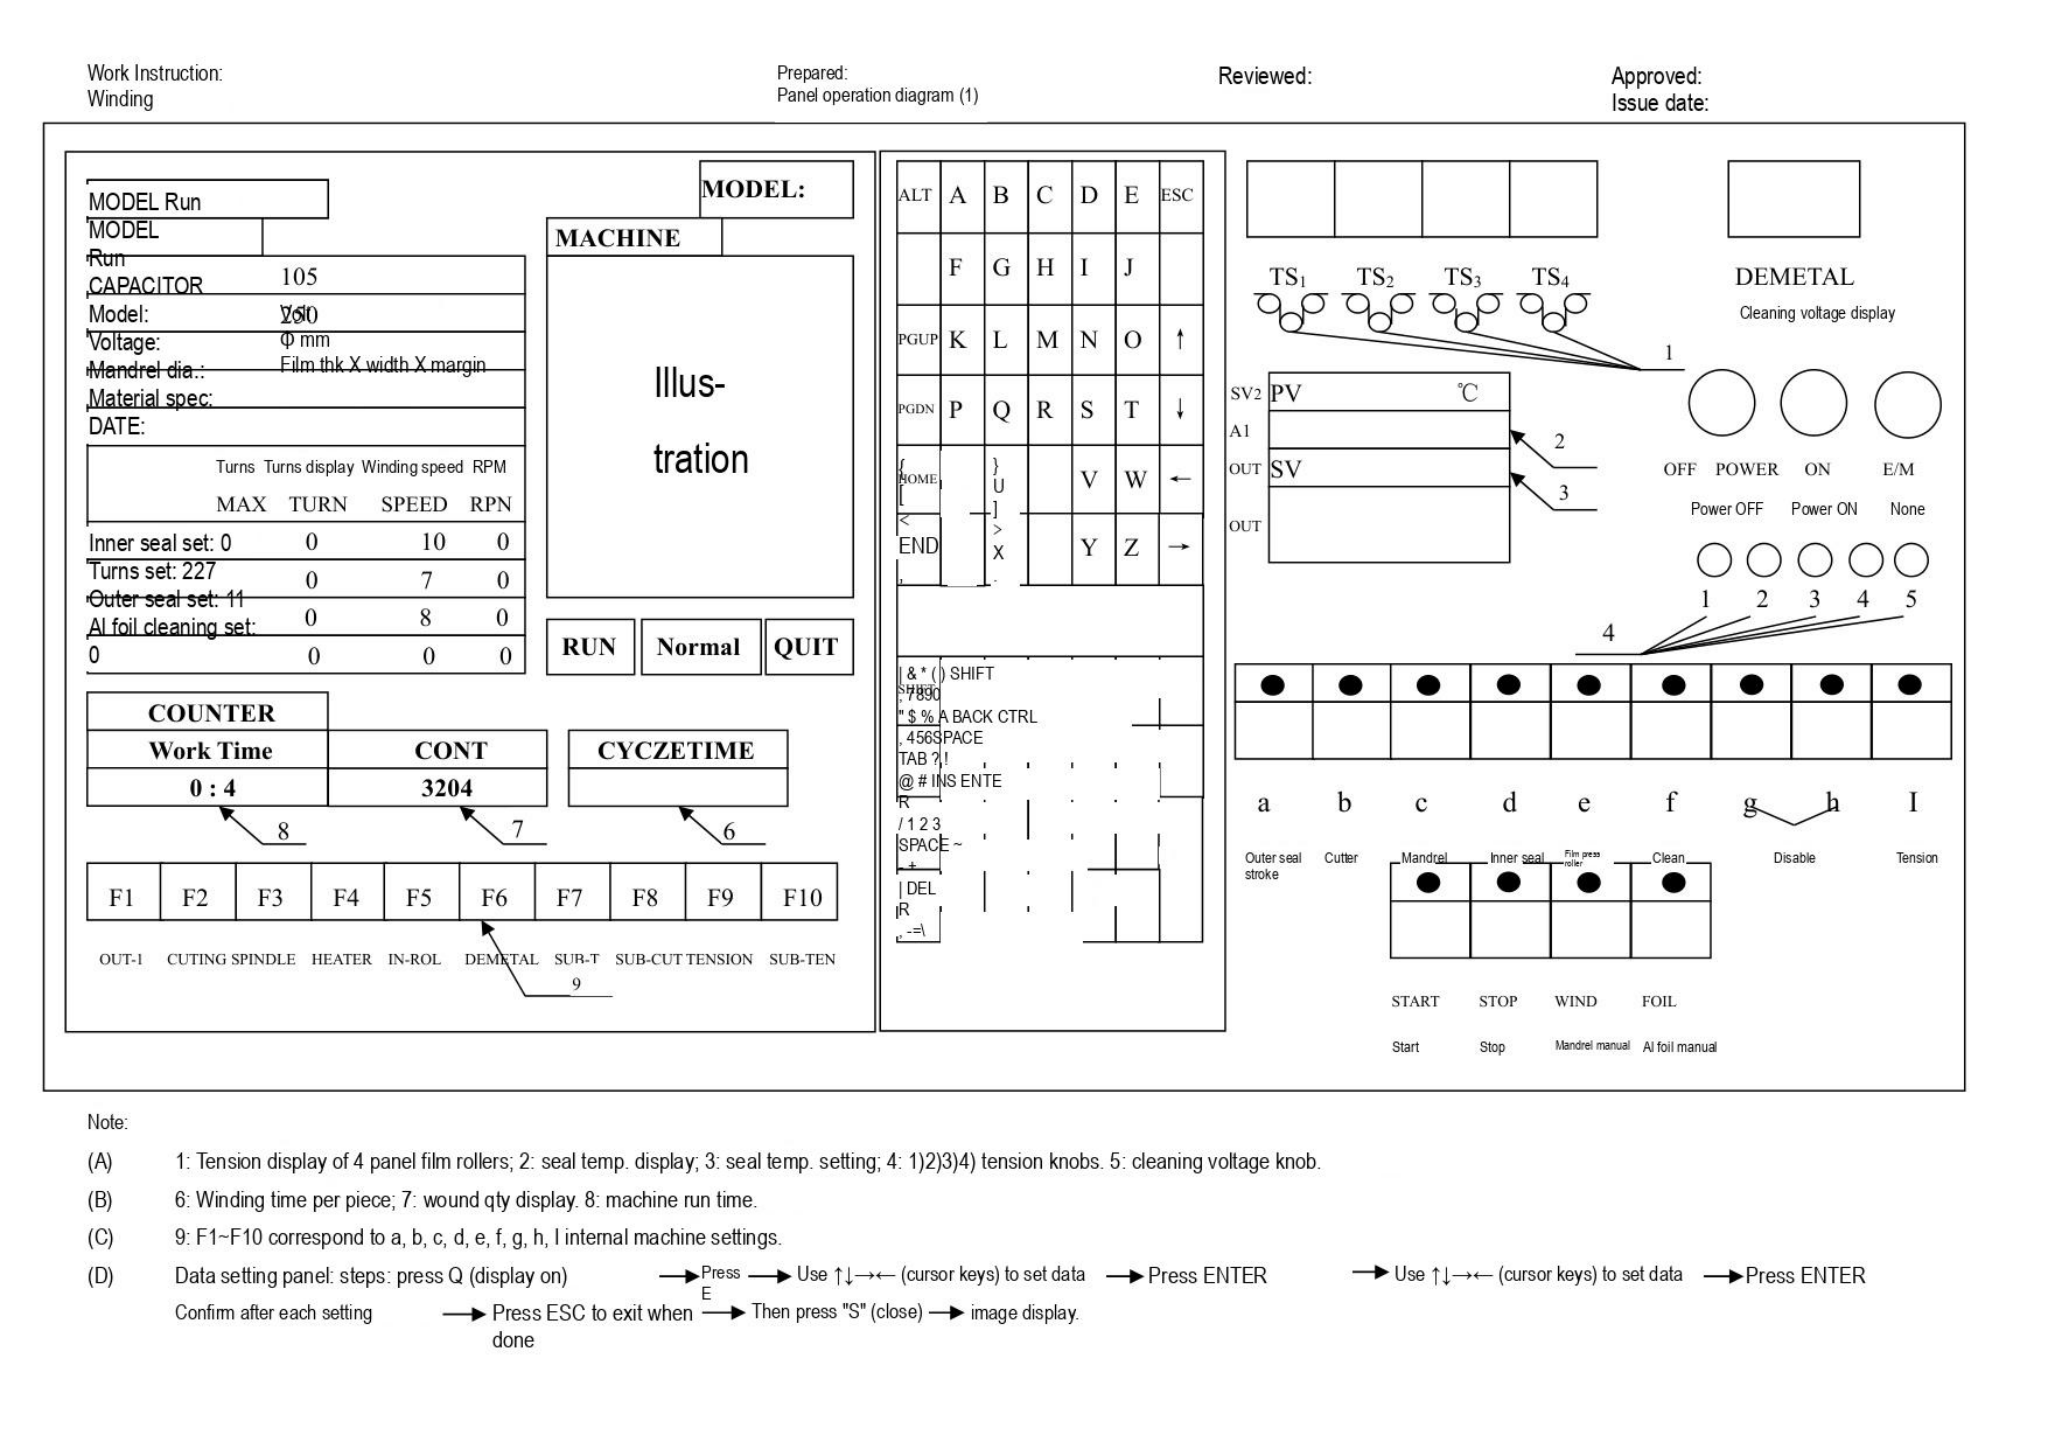Work Instruction:
Winding

Prepared:
Panel operation diagram (1)

Reviewed:

Approved:
Issue date:

MODEL Run
MODEL
Run

| | |
|---|---|
| CAPACITOR | 105 |
| Model: | 250 |
| Voltage: | Φ mm |
| Mandrel dia.: | Film thk X width X margin |
| Material spec: | |
| DATE: | |

| Turns | Turns display | Winding speed | RPM |
|---|---|---|---|
| MAX | TURN | SPEED | RPN |
| Inner seal set: 0 | 0 | 10 | 0 |
| Turns set: 227 | 0 | 7 | 0 |
| Outer seal set: 11 | 0 | 8 | 0 |
| Al foil cleaning set: | 0 | 0 | 0 |
| 0 | | | |

MODEL:

MACHINE

Illus-
tration

RUN Normal QUIT

| COUNTER | | |
|---|---|---|
| Work Time | CONT | CYCZETIME |
| 0 : 4 | 3204 | |

8 7 6

| F1 | F2 | F3 | F4 | F5 | F6 | F7 | F8 | F9 | F10 |
|---|---|---|---|---|---|---|---|---|---|

OUT-1 CUTING SPINDLE HEATER IN-ROL DEMETAL SUB-T SUB-CUT TENSION SUB-TEN

9

| ALT | A | B | C | D | E | ESC |
|---|---|---|---|---|---|---|
| | F | G | H | I | J | |
| PGUP | K | L | M | N | O | ↑ |
| PGDN | P | Q | R | S | T | ↓ |
| { HOME [ | | } U ] | | V | W | ← |
| < END | | > X | | Y | Z | → |

| & * ( ) SHIFT
SHIFT
, / 890
" $ % A BACK CTRL
, 456SPACE
TAB ? !
@ # INS ENTE
R
/ 1 2 3
SPACE ~
_ +
| DEL
R
. -=\

TS1 TS2 TS3 TS4

1

DEMETAL
Cleaning voltage display

SV2 PV ℃
A1
OUT SV
OUT

2
3

OFF POWER ON E/M
Power OFF Power ON None

1 2 3 4 5

4

a b c d e f g h I

Outer seal stroke | Cutter | Mandrel | Inner seal | Film press roller | Clean | Disable | Tension

START STOP WIND FOIL
Start Stop Mandrel manual Al foil manual

Note:

(A) 1: Tension display of 4 panel film rollers; 2: seal temp. display; 3: seal temp. setting; 4: 1)2)3)4) tension knobs. 5: cleaning voltage knob.

(B) 6: Winding time per piece; 7: wound qty display. 8: machine run time.

(C) 9: F1~F10 correspond to a, b, c, d, e, f, g, h, I internal machine settings.

(D) Data setting panel: steps: press Q (display on) → Press E → Use ↑↓→← (cursor keys) to set data → Press ENTER → Use ↑↓→← (cursor keys) to set data → Press ENTER
Confirm after each setting → Press ESC to exit when done → Then press "S" (close) → image display.
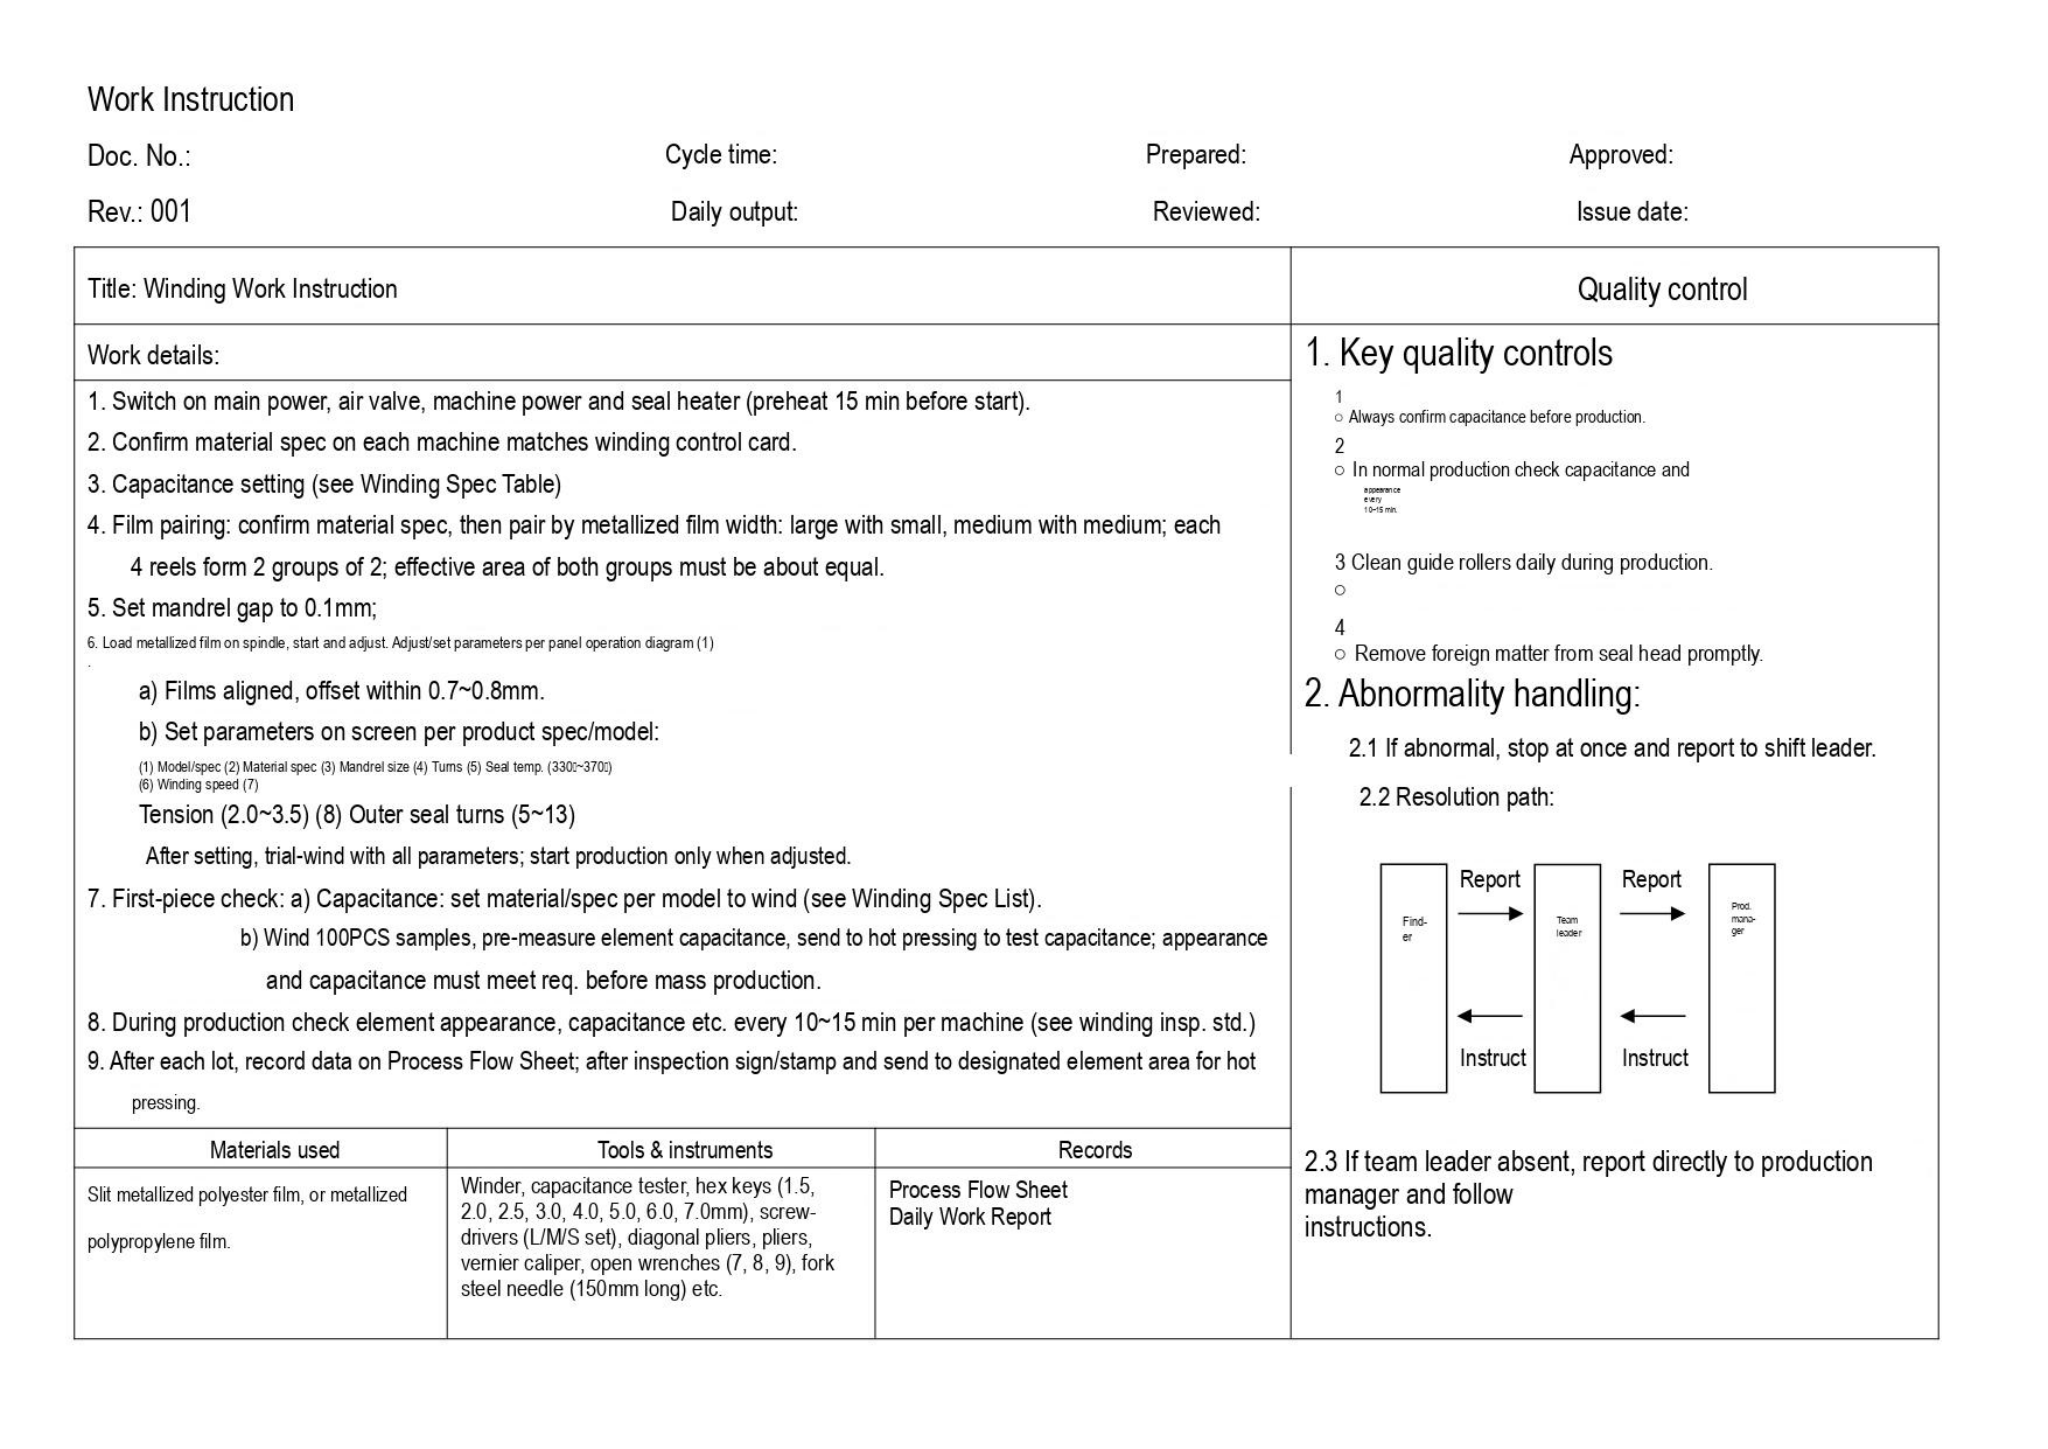Work Instruction

Doc. No.: Cycle time: Prepared: Approved:

Rev.: 001 Daily output: Reviewed: Issue date:

Title: Winding Work Instruction

Work details:

1. Switch on main power, air valve, machine power and seal heater (preheat 15 min before start).
2. Confirm material spec on each machine matches winding control card.
3. Capacitance setting (see Winding Spec Table)
4. Film pairing: confirm material spec, then pair by metallized film width: large with small, medium with medium; each 4 reels form 2 groups of 2; effective area of both groups must be about equal.
5. Set mandrel gap to 0.1mm;
6. Load metallized film on spindle, start and adjust. Adjust/set parameters per panel operation diagram (1)
   a) Films aligned, offset within 0.7~0.8mm.
   b) Set parameters on screen per product spec/model:
   (1) Model/spec (2) Material spec (3) Mandrel size (4) Turns (5) Seal temp. (330~370)
   (6) Winding speed (7)
   Tension (2.0~3.5) (8) Outer seal turns (5~13)
   After setting, trial-wind with all parameters; start production only when adjusted.
7. First-piece check: a) Capacitance: set material/spec per model to wind (see Winding Spec List).
   b) Wind 100PCS samples, pre-measure element capacitance, send to hot pressing to test capacitance; appearance and capacitance must meet req. before mass production.
8. During production check element appearance, capacitance etc. every 10~15 min per machine (see winding insp. std.)
9. After each lot, record data on Process Flow Sheet; after inspection sign/stamp and send to designated element area for hot pressing.

| Materials used | Tools & instruments | Records |
|---|---|---|
| Slit metallized polyester film, or metallized polypropylene film. | Winder, capacitance tester, hex keys (1.5, 2.0, 2.5, 3.0, 4.0, 5.0, 6.0, 7.0mm), screw-drivers (L/M/S set), diagonal pliers, pliers, vernier caliper, open wrenches (7, 8, 9), fork steel needle (150mm long) etc. | Process Flow Sheet<br>Daily Work Report |

Quality control

1. Key quality controls

1
○ Always confirm capacitance before production.

2
○ In normal production check capacitance and appearance every 10~15 min.

3 Clean guide rollers daily during production.
○

4
○ Remove foreign matter from seal head promptly.

2. Abnormality handling:

2.1 If abnormal, stop at once and report to shift leader.

2.2 Resolution path:

Finder — Report → Team leader — Report → Prod. manager

Finder ← Instruct — Team leader ← Instruct — Prod. manager

2.3 If team leader absent, report directly to production manager and follow instructions.